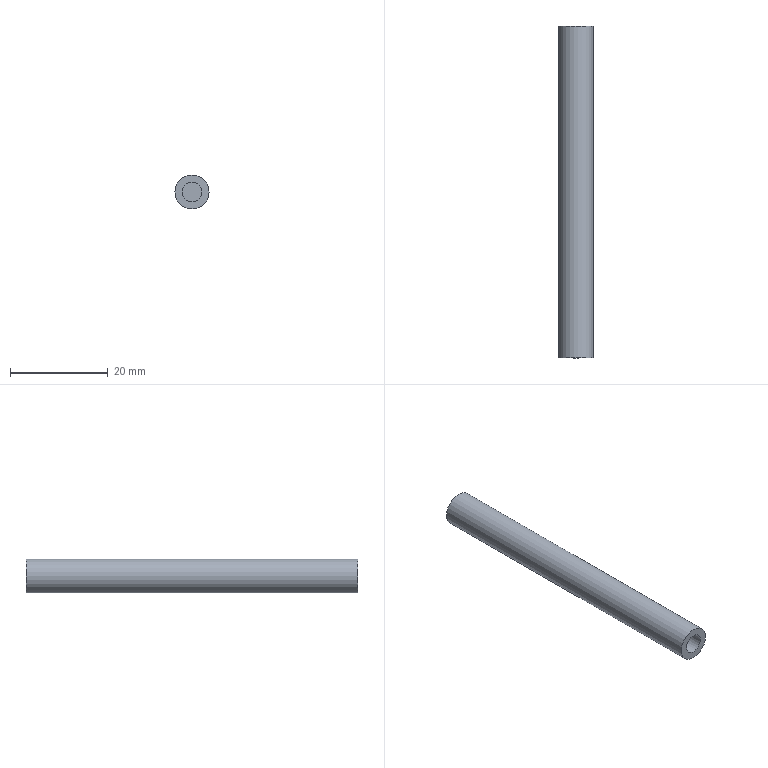Part | STEP file | 1-04.3 | 1 solid | 7 faces | box 7 x 68 x 7 mm | volume 2391 mm3 | plane 4 | cylinder 3 | commonest cylinder face diameters 4 x2 7 x1
STEP:
#1=CARTESIAN_POINT('',(0.,0.,0.));
#2=DIRECTION('',(0.,0.,1.));
#3=DIRECTION('',(1.,0.,0.));
#4=AXIS2_PLACEMENT_3D('',#1,#2,#3);
#5=CARTESIAN_POINT('',(3.5,-34.,0.));
#6=VERTEX_POINT('',#5);
#7=CARTESIAN_POINT('',(3.5,34.,0.));
#8=VERTEX_POINT('',#7);
#9=CARTESIAN_POINT('',(3.5,-34.,0.));
#10=DIRECTION('',(0.,1.,0.));
#11=VECTOR('',#10,1.);
#12=LINE('',#9,#11);
#13=CARTESIAN_POINT('',(0.,-34.,0.));
#14=DIRECTION('',(0.,1.,0.));
#15=DIRECTION('',(1.,0.,0.));
#16=AXIS2_PLACEMENT_3D('',#13,#14,#15);
#17=CYLINDRICAL_SURFACE('',#16,3.5);
#18=CARTESIAN_POINT('',(6.283,0.));
#19=DIRECTION('',(0.,1.));
#20=VECTOR('',#19,1.);
#21=LINE('',#18,#20);
#22=(GEOMETRIC_REPRESENTATION_CONTEXT(2)PARAMETRIC_REPRESENTATION_CONTEXT()REPRESENTATION_CONTEXT('',''));
#23=DEFINITIONAL_REPRESENTATION('',(#21),#22);
#24=PCURVE('',#17,#23);
#25=CARTESIAN_POINT('',(0.,0.));
#26=DIRECTION('',(0.,1.));
#27=VECTOR('',#26,1.);
#28=LINE('',#25,#27);
#29=(GEOMETRIC_REPRESENTATION_CONTEXT(2)PARAMETRIC_REPRESENTATION_CONTEXT()REPRESENTATION_CONTEXT('',''));
#30=DEFINITIONAL_REPRESENTATION('',(#28),#29);
#31=PCURVE('',#17,#30);
#32=SEAM_CURVE('',#12,(#24,#31),.PCURVE_S1.);
#33=EDGE_CURVE('',#6,#8,#32,.T.);
#34=ORIENTED_EDGE('',*,*,#33,.T.);
#35=CARTESIAN_POINT('',(0.,34.,0.));
#36=DIRECTION('',(0.,-1.,0.));
#37=DIRECTION('',(1.,0.,0.));
#38=AXIS2_PLACEMENT_3D('',#35,#36,#37);
#39=CIRCLE('',#38,3.5);
#40=CARTESIAN_POINT('',(6.283,68.));
#41=DIRECTION('',(-1.,0.));
#42=VECTOR('',#41,1.);
#43=LINE('',#40,#42);
#44=(GEOMETRIC_REPRESENTATION_CONTEXT(2)PARAMETRIC_REPRESENTATION_CONTEXT()REPRESENTATION_CONTEXT('',''));
#45=DEFINITIONAL_REPRESENTATION('',(#43),#44);
#46=PCURVE('',#17,#45);
#47=CARTESIAN_POINT('',(-0.9378,34.,0.));
#48=DIRECTION('',(0.,-1.,0.));
#49=DIRECTION('',(1.,0.,0.));
#50=AXIS2_PLACEMENT_3D('',#47,#48,#49);
#51=PLANE('',#50);
#52=CARTESIAN_POINT('',(0.9378,0.));
#53=DIRECTION('',(1.,0.));
#54=AXIS2_PLACEMENT_2D('',#52,#53);
#55=CIRCLE('',#54,3.5);
#56=(GEOMETRIC_REPRESENTATION_CONTEXT(2)PARAMETRIC_REPRESENTATION_CONTEXT()REPRESENTATION_CONTEXT('',''));
#57=DEFINITIONAL_REPRESENTATION('',(#55),#56);
#58=PCURVE('',#51,#57);
#59=SURFACE_CURVE('',#39,(#46,#58),.PCURVE_S1.);
#60=EDGE_CURVE('',#8,#8,#59,.T.);
#61=ORIENTED_EDGE('',*,*,#60,.T.);
#62=ORIENTED_EDGE('',*,*,#33,.F.);
#63=CARTESIAN_POINT('',(0.,-34.,0.));
#64=DIRECTION('',(0.,-1.,0.));
#65=DIRECTION('',(1.,0.,0.));
#66=AXIS2_PLACEMENT_3D('',#63,#64,#65);
#67=CIRCLE('',#66,3.5);
#68=CARTESIAN_POINT('',(6.283,0.));
#69=DIRECTION('',(-1.,0.));
#70=VECTOR('',#69,1.);
#71=LINE('',#68,#70);
#72=(GEOMETRIC_REPRESENTATION_CONTEXT(2)PARAMETRIC_REPRESENTATION_CONTEXT()REPRESENTATION_CONTEXT('',''));
#73=DEFINITIONAL_REPRESENTATION('',(#71),#72);
#74=PCURVE('',#17,#73);
#75=CARTESIAN_POINT('',(-0.9378,-34.,0.));
#76=DIRECTION('',(0.,-1.,0.));
#77=DIRECTION('',(1.,0.,0.));
#78=AXIS2_PLACEMENT_3D('',#75,#76,#77);
#79=PLANE('',#78);
#80=CARTESIAN_POINT('',(0.9378,0.));
#81=DIRECTION('',(1.,0.));
#82=AXIS2_PLACEMENT_2D('',#80,#81);
#83=CIRCLE('',#82,3.5);
#84=(GEOMETRIC_REPRESENTATION_CONTEXT(2)PARAMETRIC_REPRESENTATION_CONTEXT()REPRESENTATION_CONTEXT('',''));
#85=DEFINITIONAL_REPRESENTATION('',(#83),#84);
#86=PCURVE('',#79,#85);
#87=SURFACE_CURVE('',#67,(#74,#86),.PCURVE_S1.);
#88=EDGE_CURVE('',#6,#6,#87,.T.);
#89=ORIENTED_EDGE('',*,*,#88,.F.);
#90=EDGE_LOOP('',(#34,#61,#62,#89));
#91=FACE_BOUND('',#90,.T.);
#92=ADVANCED_FACE('',(#91),#17,.T.);
#93=ORIENTED_EDGE('',*,*,#88,.T.);
#94=EDGE_LOOP('',(#93));
#95=FACE_BOUND('',#94,.T.);
#96=CARTESIAN_POINT('',(2.,-34.,0.));
#97=VERTEX_POINT('',#96);
#98=CARTESIAN_POINT('',(0.,-34.,0.));
#99=DIRECTION('',(0.,-1.,0.));
#100=DIRECTION('',(1.,0.,0.));
#101=AXIS2_PLACEMENT_3D('',#98,#99,#100);
#102=CIRCLE('',#101,2.);
#103=CARTESIAN_POINT('',(0.9378,0.));
#104=DIRECTION('',(1.,0.));
#105=AXIS2_PLACEMENT_2D('',#103,#104);
#106=CIRCLE('',#105,2.);
#107=(GEOMETRIC_REPRESENTATION_CONTEXT(2)PARAMETRIC_REPRESENTATION_CONTEXT()REPRESENTATION_CONTEXT('',''));
#108=DEFINITIONAL_REPRESENTATION('',(#106),#107);
#109=PCURVE('',#79,#108);
#110=CARTESIAN_POINT('',(0.,-34.,0.));
#111=DIRECTION('',(0.,1.,0.));
#112=DIRECTION('',(1.,0.,0.));
#113=AXIS2_PLACEMENT_3D('',#110,#111,#112);
#114=CYLINDRICAL_SURFACE('',#113,2.);
#115=CARTESIAN_POINT('',(6.283,0.));
#116=DIRECTION('',(-1.,0.));
#117=VECTOR('',#116,1.);
#118=LINE('',#115,#117);
#119=(GEOMETRIC_REPRESENTATION_CONTEXT(2)PARAMETRIC_REPRESENTATION_CONTEXT()REPRESENTATION_CONTEXT('',''));
#120=DEFINITIONAL_REPRESENTATION('',(#118),#119);
#121=PCURVE('',#114,#120);
#122=SURFACE_CURVE('',#102,(#109,#121),.PCURVE_S1.);
#123=EDGE_CURVE('',#97,#97,#122,.T.);
#124=ORIENTED_EDGE('',*,*,#123,.F.);
#125=EDGE_LOOP('',(#124));
#126=FACE_BOUND('',#125,.T.);
#127=ADVANCED_FACE('',(#95,#126),#79,.T.);
#128=CARTESIAN_POINT('',(2.,-25.,0.));
#129=VERTEX_POINT('',#128);
#130=CARTESIAN_POINT('',(2.,-34.,0.));
#131=DIRECTION('',(0.,1.,0.));
#132=VECTOR('',#131,1.);
#133=LINE('',#130,#132);
#134=CARTESIAN_POINT('',(6.283,0.));
#135=DIRECTION('',(0.,1.));
#136=VECTOR('',#135,1.);
#137=LINE('',#134,#136);
#138=(GEOMETRIC_REPRESENTATION_CONTEXT(2)PARAMETRIC_REPRESENTATION_CONTEXT()REPRESENTATION_CONTEXT('',''));
#139=DEFINITIONAL_REPRESENTATION('',(#137),#138);
#140=PCURVE('',#114,#139);
#141=CARTESIAN_POINT('',(0.,0.));
#142=DIRECTION('',(0.,1.));
#143=VECTOR('',#142,1.);
#144=LINE('',#141,#143);
#145=(GEOMETRIC_REPRESENTATION_CONTEXT(2)PARAMETRIC_REPRESENTATION_CONTEXT()REPRESENTATION_CONTEXT('',''));
#146=DEFINITIONAL_REPRESENTATION('',(#144),#145);
#147=PCURVE('',#114,#146);
#148=SEAM_CURVE('',#133,(#140,#147),.PCURVE_S1.);
#149=EDGE_CURVE('',#97,#129,#148,.T.);
#150=ORIENTED_EDGE('',*,*,#149,.T.);
#151=CARTESIAN_POINT('',(0.,-25.,0.));
#152=DIRECTION('',(0.,-1.,0.));
#153=DIRECTION('',(1.,0.,0.));
#154=AXIS2_PLACEMENT_3D('',#151,#152,#153);
#155=CIRCLE('',#154,2.);
#156=CARTESIAN_POINT('',(6.283,9.));
#157=DIRECTION('',(-1.,0.));
#158=VECTOR('',#157,1.);
#159=LINE('',#156,#158);
#160=(GEOMETRIC_REPRESENTATION_CONTEXT(2)PARAMETRIC_REPRESENTATION_CONTEXT()REPRESENTATION_CONTEXT('',''));
#161=DEFINITIONAL_REPRESENTATION('',(#159),#160);
#162=PCURVE('',#114,#161);
#163=CARTESIAN_POINT('',(-0.5359,-25.,0.));
#164=DIRECTION('',(0.,-1.,0.));
#165=DIRECTION('',(1.,0.,0.));
#166=AXIS2_PLACEMENT_3D('',#163,#164,#165);
#167=PLANE('',#166);
#168=CARTESIAN_POINT('',(0.5359,0.));
#169=DIRECTION('',(1.,0.));
#170=AXIS2_PLACEMENT_2D('',#168,#169);
#171=CIRCLE('',#170,2.);
#172=(GEOMETRIC_REPRESENTATION_CONTEXT(2)PARAMETRIC_REPRESENTATION_CONTEXT()REPRESENTATION_CONTEXT('',''));
#173=DEFINITIONAL_REPRESENTATION('',(#171),#172);
#174=PCURVE('',#167,#173);
#175=SURFACE_CURVE('',#155,(#162,#174),.PCURVE_S1.);
#176=EDGE_CURVE('',#129,#129,#175,.T.);
#177=ORIENTED_EDGE('',*,*,#176,.T.);
#178=ORIENTED_EDGE('',*,*,#149,.F.);
#179=ORIENTED_EDGE('',*,*,#123,.F.);
#180=EDGE_LOOP('',(#150,#177,#178,#179));
#181=FACE_BOUND('',#180,.F.);
#182=ADVANCED_FACE('',(#181),#114,.F.);
#183=ORIENTED_EDGE('',*,*,#176,.T.);
#184=EDGE_LOOP('',(#183));
#185=FACE_BOUND('',#184,.T.);
#186=ADVANCED_FACE('',(#185),#167,.T.);
#187=ORIENTED_EDGE('',*,*,#60,.T.);
#188=EDGE_LOOP('',(#187));
#189=FACE_BOUND('',#188,.F.);
#190=CARTESIAN_POINT('',(2.,34.,0.));
#191=VERTEX_POINT('',#190);
#192=CARTESIAN_POINT('',(0.,34.,0.));
#193=DIRECTION('',(0.,-1.,0.));
#194=DIRECTION('',(1.,0.,0.));
#195=AXIS2_PLACEMENT_3D('',#192,#193,#194);
#196=CIRCLE('',#195,2.);
#197=CARTESIAN_POINT('',(0.9378,0.));
#198=DIRECTION('',(1.,0.));
#199=AXIS2_PLACEMENT_2D('',#197,#198);
#200=CIRCLE('',#199,2.);
#201=(GEOMETRIC_REPRESENTATION_CONTEXT(2)PARAMETRIC_REPRESENTATION_CONTEXT()REPRESENTATION_CONTEXT('',''));
#202=DEFINITIONAL_REPRESENTATION('',(#200),#201);
#203=PCURVE('',#51,#202);
#204=CARTESIAN_POINT('',(0.,34.,0.));
#205=DIRECTION('',(0.,-1.,0.));
#206=DIRECTION('',(1.,0.,0.));
#207=AXIS2_PLACEMENT_3D('',#204,#205,#206);
#208=CYLINDRICAL_SURFACE('',#207,2.);
#209=CARTESIAN_POINT('',(0.,0.));
#210=DIRECTION('',(1.,0.));
#211=VECTOR('',#210,1.);
#212=LINE('',#209,#211);
#213=(GEOMETRIC_REPRESENTATION_CONTEXT(2)PARAMETRIC_REPRESENTATION_CONTEXT()REPRESENTATION_CONTEXT('',''));
#214=DEFINITIONAL_REPRESENTATION('',(#212),#213);
#215=PCURVE('',#208,#214);
#216=SURFACE_CURVE('',#196,(#203,#215),.PCURVE_S1.);
#217=EDGE_CURVE('',#191,#191,#216,.T.);
#218=ORIENTED_EDGE('',*,*,#217,.F.);
#219=EDGE_LOOP('',(#218));
#220=FACE_BOUND('',#219,.F.);
#221=ADVANCED_FACE('',(#189,#220),#51,.F.);
#222=ORIENTED_EDGE('',*,*,#217,.T.);
#223=CARTESIAN_POINT('',(2.,25.,0.));
#224=VERTEX_POINT('',#223);
#225=CARTESIAN_POINT('',(2.,34.,0.));
#226=DIRECTION('',(0.,-1.,0.));
#227=VECTOR('',#226,1.);
#228=LINE('',#225,#227);
#229=CARTESIAN_POINT('',(6.283,0.));
#230=DIRECTION('',(0.,1.));
#231=VECTOR('',#230,1.);
#232=LINE('',#229,#231);
#233=(GEOMETRIC_REPRESENTATION_CONTEXT(2)PARAMETRIC_REPRESENTATION_CONTEXT()REPRESENTATION_CONTEXT('',''));
#234=DEFINITIONAL_REPRESENTATION('',(#232),#233);
#235=PCURVE('',#208,#234);
#236=CARTESIAN_POINT('',(0.,0.));
#237=DIRECTION('',(0.,1.));
#238=VECTOR('',#237,1.);
#239=LINE('',#236,#238);
#240=(GEOMETRIC_REPRESENTATION_CONTEXT(2)PARAMETRIC_REPRESENTATION_CONTEXT()REPRESENTATION_CONTEXT('',''));
#241=DEFINITIONAL_REPRESENTATION('',(#239),#240);
#242=PCURVE('',#208,#241);
#243=SEAM_CURVE('',#228,(#235,#242),.PCURVE_S1.);
#244=EDGE_CURVE('',#191,#224,#243,.T.);
#245=ORIENTED_EDGE('',*,*,#244,.T.);
#246=CARTESIAN_POINT('',(0.,25.,0.));
#247=DIRECTION('',(0.,-1.,0.));
#248=DIRECTION('',(1.,0.,0.));
#249=AXIS2_PLACEMENT_3D('',#246,#247,#248);
#250=CIRCLE('',#249,2.);
#251=CARTESIAN_POINT('',(0.,9.));
#252=DIRECTION('',(1.,0.));
#253=VECTOR('',#252,1.);
#254=LINE('',#251,#253);
#255=(GEOMETRIC_REPRESENTATION_CONTEXT(2)PARAMETRIC_REPRESENTATION_CONTEXT()REPRESENTATION_CONTEXT('',''));
#256=DEFINITIONAL_REPRESENTATION('',(#254),#255);
#257=PCURVE('',#208,#256);
#258=CARTESIAN_POINT('',(-0.5359,25.,0.));
#259=DIRECTION('',(0.,-1.,0.));
#260=DIRECTION('',(1.,0.,0.));
#261=AXIS2_PLACEMENT_3D('',#258,#259,#260);
#262=PLANE('',#261);
#263=CARTESIAN_POINT('',(0.5359,0.));
#264=DIRECTION('',(1.,0.));
#265=AXIS2_PLACEMENT_2D('',#263,#264);
#266=CIRCLE('',#265,2.);
#267=(GEOMETRIC_REPRESENTATION_CONTEXT(2)PARAMETRIC_REPRESENTATION_CONTEXT()REPRESENTATION_CONTEXT('',''));
#268=DEFINITIONAL_REPRESENTATION('',(#266),#267);
#269=PCURVE('',#262,#268);
#270=SURFACE_CURVE('',#250,(#257,#269),.PCURVE_S1.);
#271=EDGE_CURVE('',#224,#224,#270,.T.);
#272=ORIENTED_EDGE('',*,*,#271,.F.);
#273=ORIENTED_EDGE('',*,*,#244,.F.);
#274=EDGE_LOOP('',(#222,#245,#272,#273));
#275=FACE_BOUND('',#274,.F.);
#276=ADVANCED_FACE('',(#275),#208,.F.);
#277=ORIENTED_EDGE('',*,*,#271,.T.);
#278=EDGE_LOOP('',(#277));
#279=FACE_BOUND('',#278,.F.);
#280=ADVANCED_FACE('',(#279),#262,.F.);
#281=CLOSED_SHELL('',(#92,#127,#182,#186,#221,#276,#280));
#282=MANIFOLD_SOLID_BREP('',#281);
#283=(LENGTH_UNIT()NAMED_UNIT(*)SI_UNIT(.MILLI.,.METRE.));
#284=UNCERTAINTY_MEASURE_WITH_UNIT(LENGTH_MEASURE(0.0000001),#283,'','');
#285=(NAMED_UNIT(*)PLANE_ANGLE_UNIT()SI_UNIT($,.RADIAN.));
#286=(NAMED_UNIT(*)SI_UNIT($,.STERADIAN.)SOLID_ANGLE_UNIT());
#287=(GEOMETRIC_REPRESENTATION_CONTEXT(3)GLOBAL_UNCERTAINTY_ASSIGNED_CONTEXT((#284))GLOBAL_UNIT_ASSIGNED_CONTEXT((#283,#285,#286))REPRESENTATION_CONTEXT('',''));
#288=ADVANCED_BREP_SHAPE_REPRESENTATION('',(#4,#282),#287);